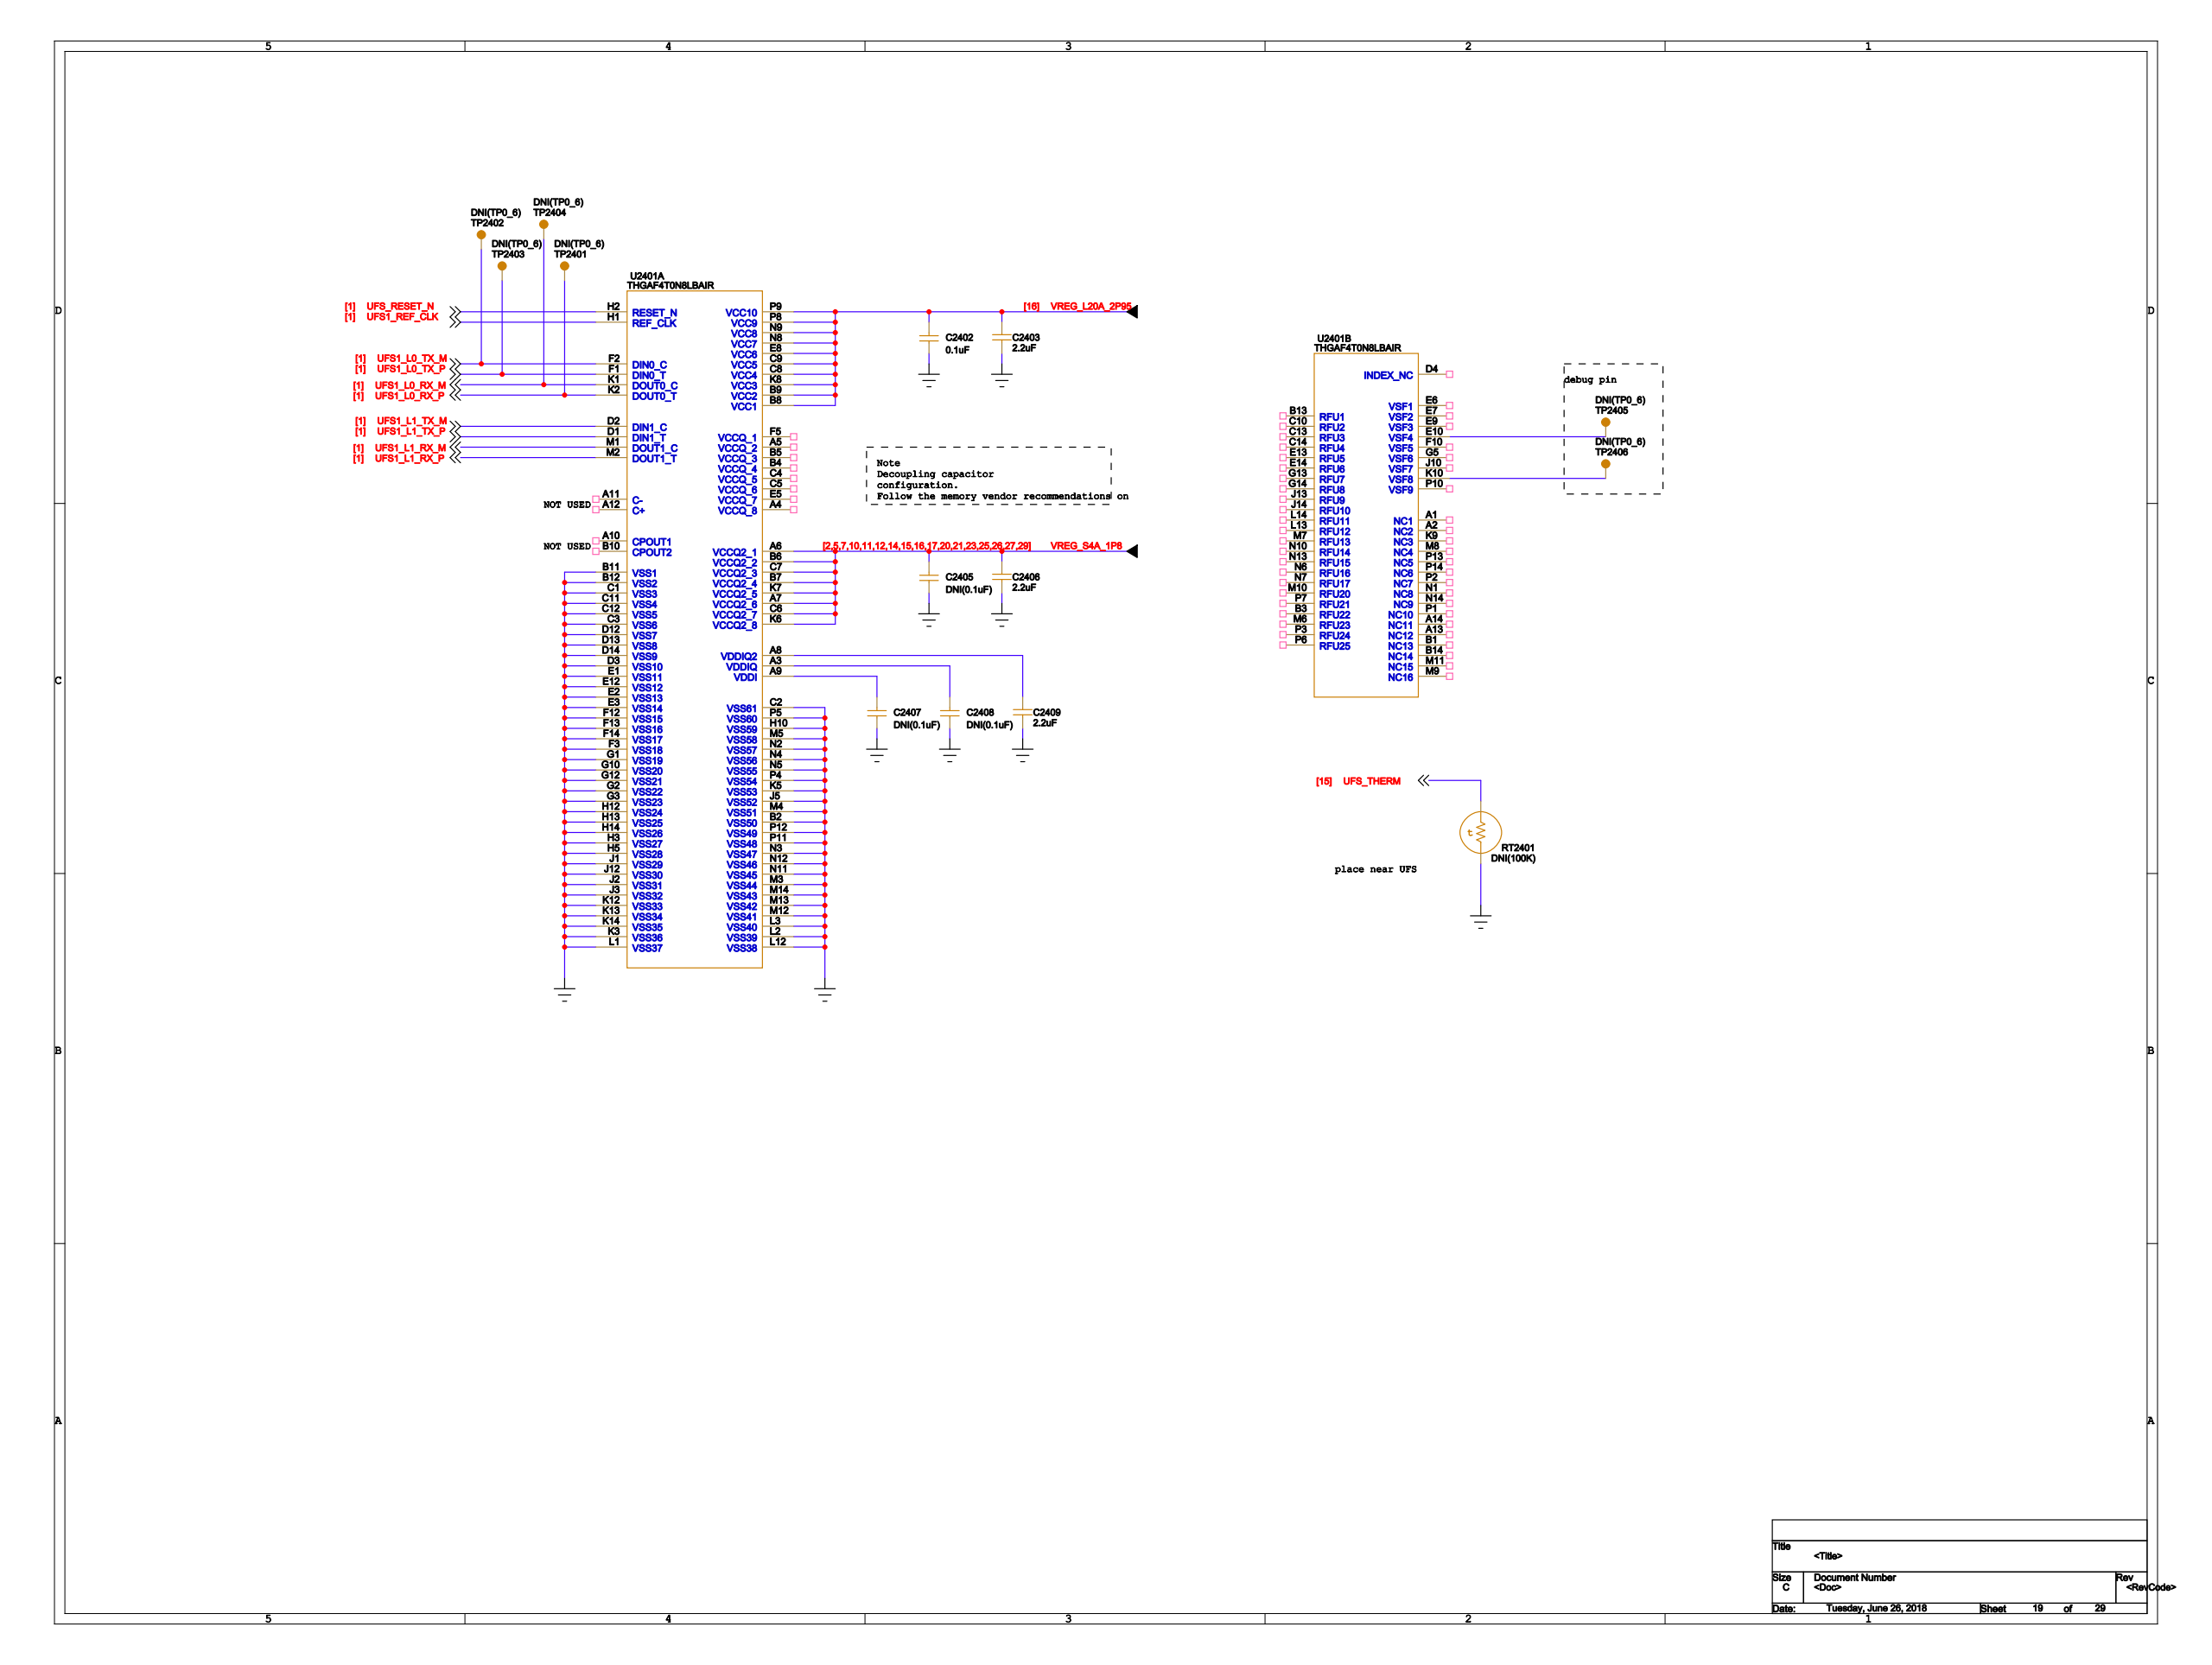Circuit board | Cadence Allegro | 802 parts | 566 nets | one sheet of the schematic
Parts on this sheet (reference | value | footprint):
C2402 | 0.1uF | C0402
C2403 | 2.2uF | 0402-BIG
C2405 | DNI(0.1uF) | C0402
C2406 | 2.2uF | 0402-BIG
C2407 | DNI(0.1uF) | C0402
C2408 | DNI(0.1uF) | C0402
C2409 | 2.2uF | 0402-BIG
J1 | SD-105435 | USB_SD-105435
RT2401 | DNI(100K) | R0402
TP2401 | DNI(TP0_6) | TP_C0P6
TP2402 | DNI(TP0_6) | TP_C0P6
TP2403 | DNI(TP0_6) | TP_C0P6
TP2404 | DNI(TP0_6) | TP_C0P6
TP2405 | DNI(TP0_6) | TP_C0P6
TP2406 | DNI(TP0_6) | TP_C0P6
U2401 | THGAF4T0N8LBAIR | FBGA153_11P5X13X1P1_0P5
Nets of these parts (net: part-pin ...):
GND: C2402-1 C2403-2 C2405-1 C2406-2 C2407-1 C2408-1 C2409-2 RT2401-2 J1-A1 J1-A12 J1-B1 J1-B12 J1-C1 J1-C2 J1-C3 J1-C4 U2401-B2 U2401-B11 U2401-B12 U2401-C1 U2401-C2 U2401-C3 U2401-C11 U2401-C12 U2401-D3 U2401-D12 U2401-D13 U2401-D14 U2401-E1 U2401-E2 U2401-E3 U2401-E12 U2401-F3 U2401-F12 U2401-F13 U2401-F14 U2401-G1 U2401-G2 U2401-G3 U2401-G10 U2401-G12 U2401-H3 U2401-H5 U2401-H10 U2401-H12 U2401-H13 U2401-H14 U2401-J1 U2401-J2 U2401-J3 U2401-J5 U2401-J12 U2401-K3 U2401-K5 U2401-K12 U2401-K13 U2401-K14 U2401-L1 U2401-L2 U2401-L3 U2401-L12 U2401-M3 U2401-M4 U2401-M5 U2401-M12 U2401-M13 U2401-M14 U2401-N2 U2401-N3 U2401-N4 U2401-N5 U2401-N11 U2401-N12 U2401-P4 U2401-P5 U2401-P11 U2401-P12
VREG_L20A_2P95: C2402-2 C2403-1 U2401-B8 U2401-B9 U2401-C8 U2401-C9 U2401-E8 U2401-K8 U2401-N8 U2401-N9 U2401-P8 U2401-P9
VREG_S4A_1P8: C2405-2 C2406-1 U2401-A6 U2401-A7 U2401-B6 U2401-B7 U2401-C6 U2401-C7 U2401-K6 U2401-K7
N398967: C2409-1 U2401-A8
N398482: C2407-2 U2401-A9
N398489: C2408-2 U2401-A3
UFS_THERM: RT2401-1
UFS1_L0_RX_P: TP2401-1 U2401-K2
UFS1_L0_TX_M: TP2402-1 U2401-F2
UFS1_L0_TX_P: TP2403-1 U2401-F1
UFS1_L0_RX_M: TP2404-1 U2401-K1
N393151: TP2405-1 U2401-E10
N393210: TP2406-1 U2401-K10
UFS1_L1_RX_M: U2401-M1
UFS1_L1_RX_P: U2401-M2
UFS1_L1_TX_M: U2401-D2
UFS1_L1_TX_P: U2401-D1
UFS1_REF_CLK: U2401-H1
UFS_RESET_N: U2401-H2